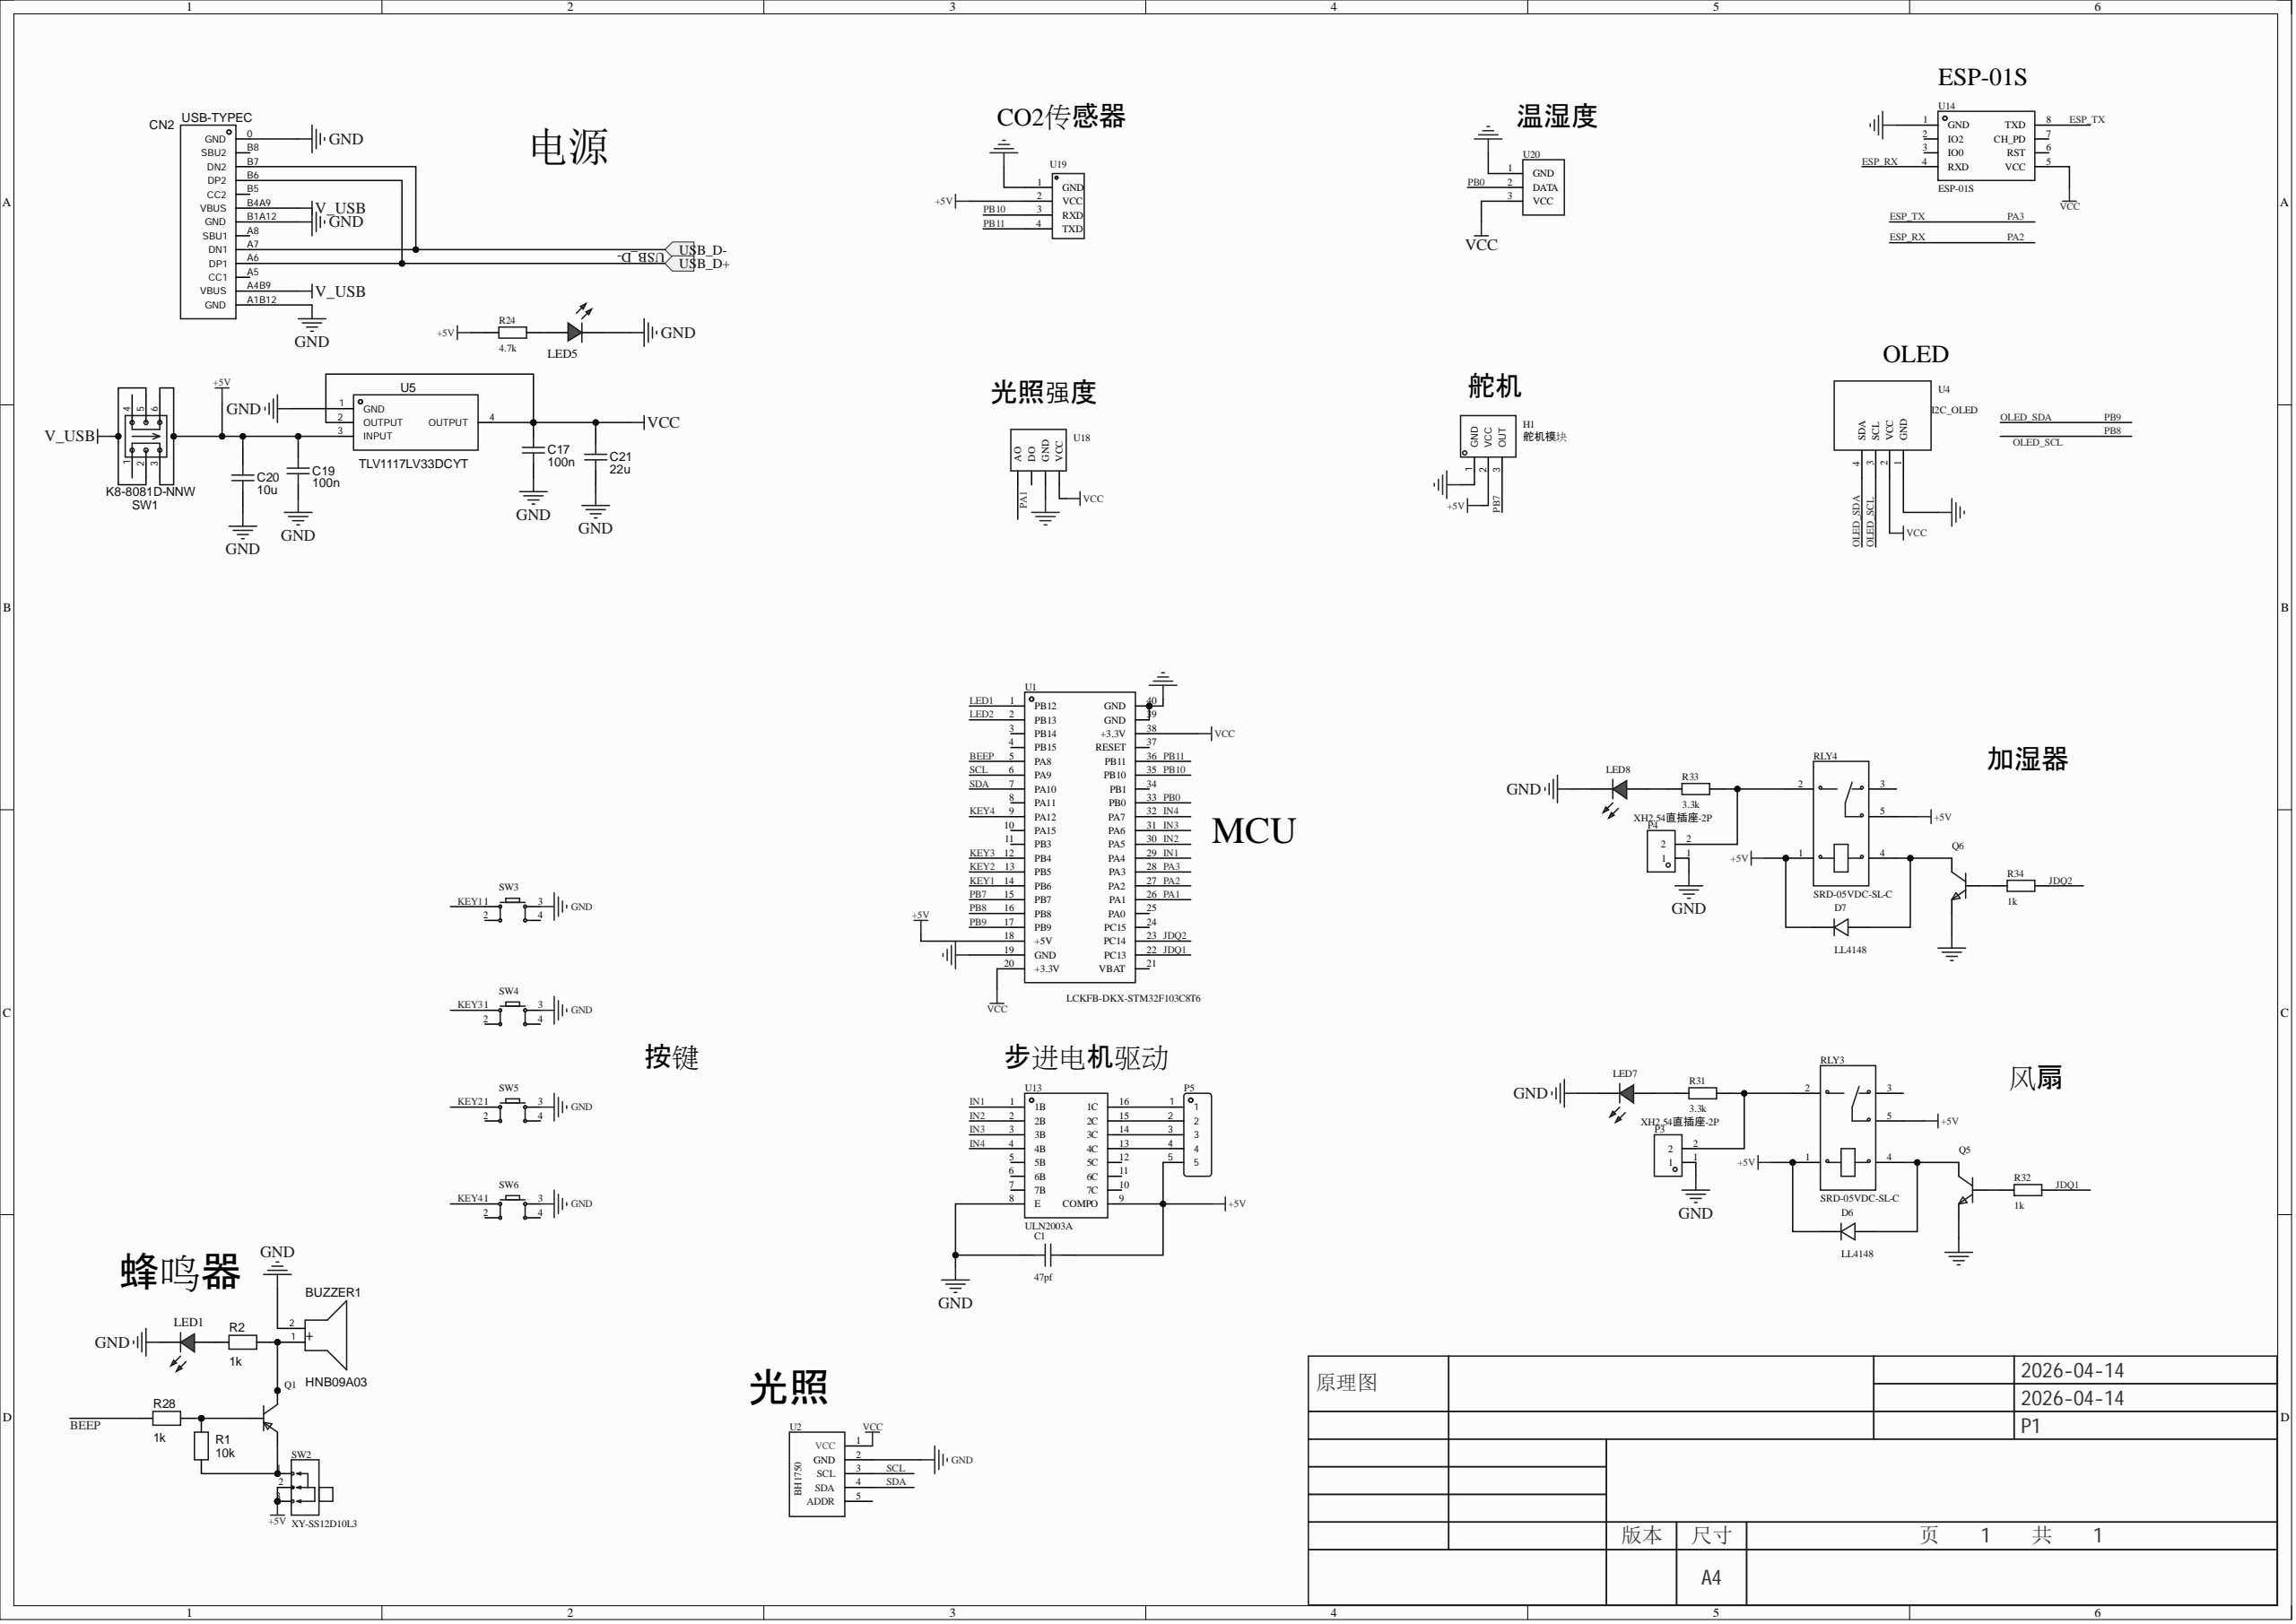Circuit board | Altium Designer | 45 parts | 45 nets
Bill of materials:
Comment,Description,Designator,Footprint,LibRef,Quantity
"HNB09A03","","BUZZER1","BUZ-TH_BD9.0-P5.00-D0.6-FD","HNB09A03","1"
"47pf","","C1","C0603","CAP_0603","1"
"100n","","C17, C19","C0603","100n","2"
"10u","","C20","C0603","100n","1"
"22u","","C21","C0603","100n","1"
"USB-TYPEC","","CN2","USB-C-SMD_MC-307","MC-307","1"
"LL4148","二极管配置:-;功率:500mW;直流反向耐压(Vr):75V;平均整流电流(Io):200mA;正向压降(Vf):1V@10mA;反向电流(Ir):5uA@75V;反向恢复时间(trr):4ns;工作温度:+175℃@(Tj);","D6, D7","LL-34_L3.5-W1.5-RD","LL4148_C9808","2"
"舵机模块","","H1","舵机模块","舵机模块","1"
"","","LED1, LED5","LED_0603","LED_0603-R","2"
"","","LED7, LED8","LED_TH-3mm","LED_TH-R_3mm","2"
"XH2.54直插座-2P","","P3, P4","CONN-TH_XH2.54-2P","XH2.54直插座-2P","2"
"","","P5","CONN-TH_XH2.54-5P","XH2.54-5P","1"
"","","Q1","S8550P_SOT","S8550_SOT_PNP","1"
"","","Q5, Q6","S8050_SOT-23","S8050_SOT_NPN","2"
"10k","","R1","R0603","1k","1"
"1k","","R2, R28, R32, R34","R0603","1k, Res_0603","4"
"4.7k","","R24","R0805","0805W8F1002T5E_C17414","1"
"3.3k","","R31, R33","R0603","Res_0603","2"
"SRD-05VDC-SL-C","线圈电压:5V;触点形式:一组转换:1C(单刀双掷-转换);触点容量(电阻负载):-;最大切换电压:250V@AC;最大切换电流:15A;","RLY3, RLY4","RELAY-TH_SRD-XXVDC-XL-C","SRD-05VDC-SL-C","2"
"K8-8081D-NNW","","SW1","SW-TH_6P-L8.0-W8.0-P2.50","XKB8080-Z","1"
"XY-SS12D10L3","拨动开关,立式直脚两档,插件,单排正拨,柄长3mm","SW2","SW-TH_3P-L12.7-W6.7_XY-SS12D10LXX","XY-SS12D10L3","1"
"","","SW3, SW4, SW5, SW6","SW-TH_4P-L6.0-W6.0-P4.50-LS6.5","Key_TH_6x6x6","4"
"LCKFB-DKX-STM32F103C8T6","","U1","CONN-TH_L53.3-W22.9_STM32F103C8T6-CARD","LCKFB-DKX-STM32F103C8T6","1"
"","","U2","BH1750光照传感器","BH1750光照传感器","1"
"","","U4","OLED_I2C_0.96","I2C_OLED","1"
"TLV1117LV33DCYT","","U5","SOT-223-4_L6.5-W3.5-P2.30-LS7.0-BR","TLV1117LV33DCYT","1"
"ULN2003A","通道数:七路;集射击穿电压(Vceo):50V;","U13","SOP-16_L10.0-W3.9-P1.27-LS6.0-BL","ULN2003A_C482013","1"
"ESP-01S","","U14","WIFIM-TH_ESP-01S","ESP-01S_C111009","1"
"光照强度模块","","U18","光敏传感器","光照强度模块","1"
"","","U19","4P排母","二氧化碳传感器","1"
"","","U20","dht11温湿度传感器","DHT11","1"
Netlist (Protel format):
[
BUZZER1
BUZ-TH_BD9.0-P5.00-D0.6-FD
HNB09A03



]
[
C1
C0603
47pf



]
[
C17
C0603
100n



]
[
C19
C0603
100n



]
[
C20
C0603
10u



]
[
C21
C0603
22u



]
[
CN2
USB-C-SMD_MC-307
USB-TYPEC



]
[
D6
LL-34_L3.5-W1.5-RD
LL4148



]
[
D7
LL-34_L3.5-W1.5-RD
LL4148



]
[
H1
舵机模块
舵机模块



]
[
LED1
LED_0603




]
[
LED5
LED_0603




]
[
LED7
LED_TH-3mm




]
[
LED8
LED_TH-3mm




]
[
P3
CONN-TH_XH2.54-2P
XH2.54直插座-2P



]
[
P4
CONN-TH_XH2.54-2P
XH2.54直插座-2P



]
[
P5
CONN-TH_XH2.54-5P




]
[
Q1
S8550P_SOT




]
[
Q5
S8050_SOT-23




]
[
Q6
S8050_SOT-23




]
[
R1
R0603
10k



]
[
R2
R0603
1k



]
[
R24
R0805
4.7k



]
[
R28
R0603
1k



]
[
R31
R0603
3.3k



]
[
R32
R0603
1k



]
[
R33
R0603
3.3k



]
[
R34
R0603
1k



]
[
RLY3
RELAY-TH_SRD-XXVDC-XL-C
SRD-05VDC-SL-C



]
[
RLY4
RELAY-TH_SRD-XXVDC-XL-C
SRD-05VDC-SL-C



]
[
SW1
SW-TH_6P-L8.0-W8.0-P2.50
K8-8081D-NNW



]
[
SW2
SW-TH_3P-L12.7-W6.7_XY-SS12D10LXX
XY-SS12D10L3



]
[
SW3
SW-TH_4P-L6.0-W6.0-P4.50-LS6.5




]
[
SW4
SW-TH_4P-L6.0-W6.0-P4.50-LS6.5




]
[
SW5
SW-TH_4P-L6.0-W6.0-P4.50-LS6.5




]
[
SW6
SW-TH_4P-L6.0-W6.0-P4.50-LS6.5




]
[
U1
CONN-TH_L53.3-W22.9_STM32F103C8T6-CARD
LCKFB-DKX-STM32F103C8T6



]
[
U2
BH1750光照传感器




]
[
U4
OLED_I2C_0.96




]
[
U5
SOT-223-4_L6.5-W3.5-P2.30-LS7.0-BR
TLV1117LV33DCYT



]
[
U13
SOP-16_L10.0-W3.9-P1.27-LS6.0-BL
ULN2003A



]
[
U14
WIFIM-TH_ESP-01S
ESP-01S



]
[
U18
光敏传感器
光照强度模块



]
[
U19
4P排母




]
[
U20
dht11温湿度传感器




]
(
VCC
C17-2
C21-2
U1-20
U1-38
U2-1
U4-2
U5-2
U5-4
U14-5
U18-1
U20-3
)
(
V_USB
CN2-A4B9
CN2-B4A9
SW1-2
SW1-5
)
(
USB_D-
CN2-A7
CN2-B7
)
(
SDA
U1-7
U2-4
)
(
SCL
U1-6
U2-3
)
(
PB11
U1-36
U19-4
)
(
PB10
U1-35
U19-3
)
(
PB7
H1-3
U1-15
)
(
PB0
U1-33
U20-2
)
(
PA1
U1-26
U18-4
)
(
OLED_SDA
U1-17
U4-4
)
(
OLED_SCL
U1-16
U4-3
)
(
NetQ6_1
Q6-1
R34-2
)
(
NetQ5_1
Q5-1
R32-2
)
(
NetQ1_2
Q1-2
R1-1
SW2-1
)
(
NetQ1_1
Q1-1
R1-2
R28-2
)
(
NetP5_4
P5-4
U13-13
)
(
NetP5_3
P5-3
U13-14
)
(
NetP5_2
P5-2
U13-15
)
(
NetP5_1
P5-1
U13-16
)
(
NetP4_2
P4-2
R33-1
RLY4-2
)
(
NetP3_2
P3-2
R31-1
RLY3-2
)
(
NetLED8_1
LED8-1
R33-2
)
(
NetLED7_1
LED7-1
R31-2
)
(
NetLED5_2
LED5-2
R24-2
)
(
NetLED1_2
LED1-2
R2-1
)
(
NetD7_2
D7-2
Q6-3
RLY4-4
)
(
NetD6_2
D6-2
Q5-3
RLY3-4
)
(
NetCN2_A6
CN2-A6
CN2-B6
)
(
NetBUZZER1_1
BUZZER1-1
Q1-3
R2-2
)
(
KEY4
SW6-1
U1-9
)
(
KEY3
SW4-1
U1-12
)
(
KEY2
SW5-1
U1-13
)
(
KEY1
SW3-1
U1-14
)
(
JDQ2
R34-1
U1-23
)
(
JDQ1
R32-1
U1-22
)
(
IN4
U1-32
U13-4
)
(
IN3
U1-31
U13-3
)
(
IN2
U1-30
U13-2
)
(
IN1
U1-29
U13-1
)
(
GND
BUZZER1-2
C1-1
C17-1
C19-1
C20-1
C21-1
CN2-0
CN2-A1B12
CN2-B1A12
H1-1
LED1-1
LED5-1
LED7-2
LED8-2
P3-1
P4-1
Q5-2
Q6-2
SW3-3
SW4-3
SW5-3
SW6-3
U1-19
U1-39
U1-40
U2-2
U4-1
U5-1
U13-8
U14-1
U18-2
U19-1
U20-1
)
(
ESP_TX
U1-28
U14-8
)
(
ESP_RX
U1-27
U14-4
)
(
BEEP
R28-1
U1-5
)
(
+5V
C1-2
C19-2
C20-2
D6-1
D7-1
H1-2
P5-5
R24-1
RLY3-1
RLY3-5
RLY4-1
RLY4-5
SW1-3
SW1-6
SW2-2
SW2-3
U1-18
U5-3
U13-9
U19-2
)